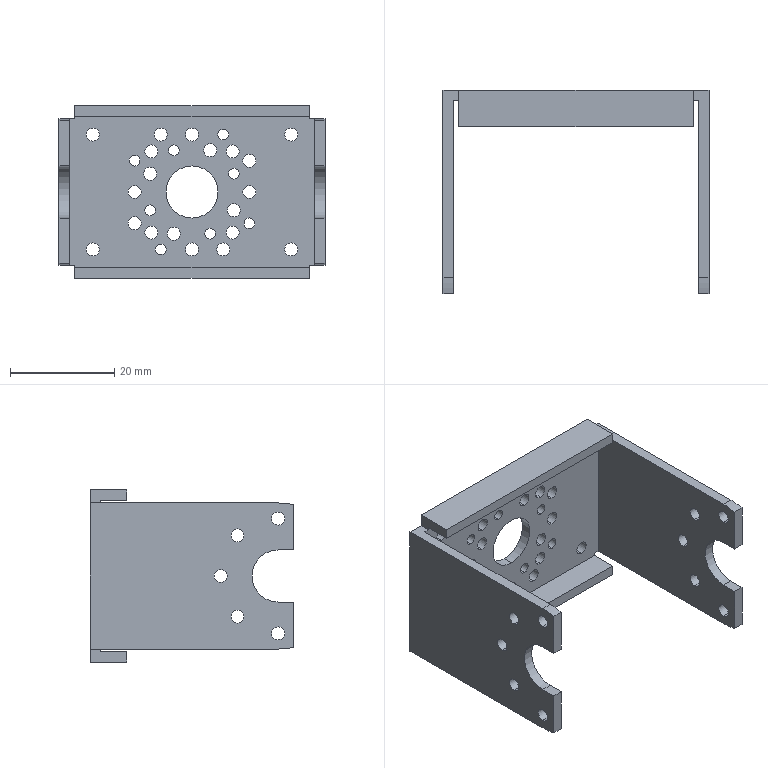Part | SolidWorks | features BaseBody 1 | 1 solid | 112 faces | box 51 x 39 x 33 mm | volume 7566 mm3 | cylinder 84 | plane 28 | commonest cylinder face diameters 2.5 x60 2.05 x16 10 x4 28 x4